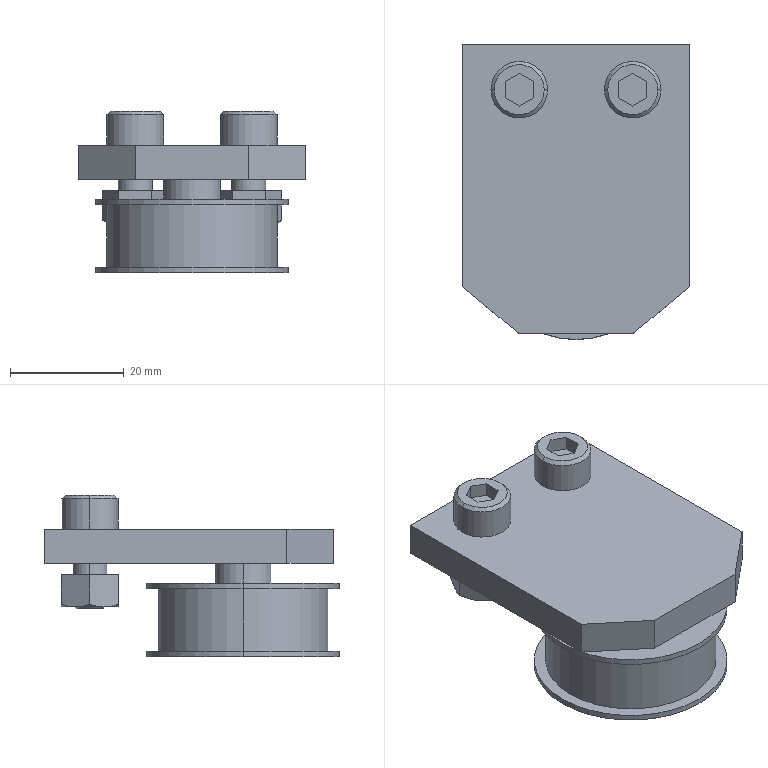Part | STEP file | ASND-0110-Q23 | 1 solid | 94 faces | box 40 x 52 x 28.5 mm | volume 23081 mm3 | plane 52 | cone 22 | cylinder 20 | commonest cylinder face diameters 10 x6 6 x4 34 x4 12 x2 17 x2 30 x2